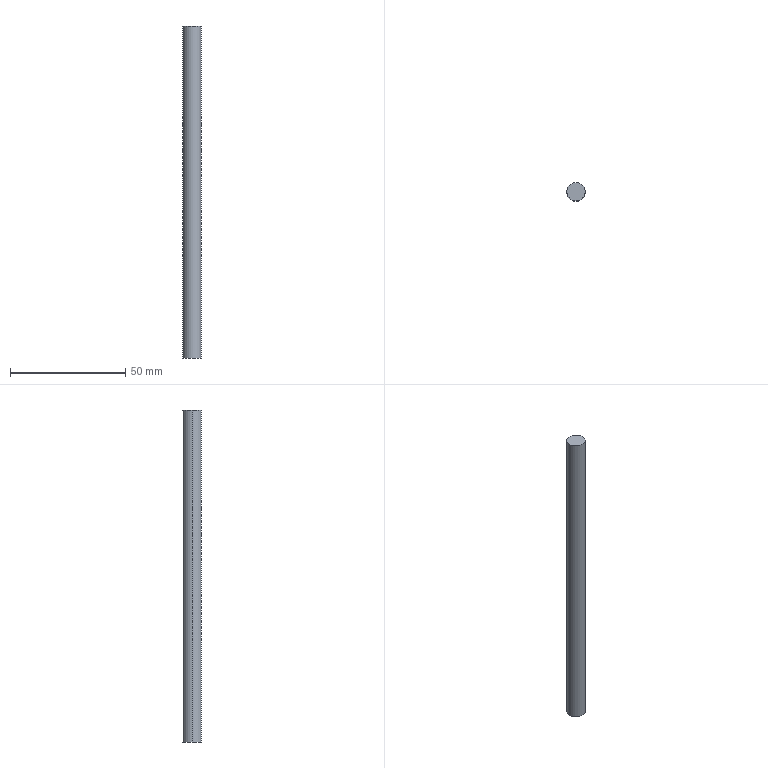Part | SolidWorks | features Extrusion 1 | 1 solid | 4 faces | box 8 x 8 x 144 mm | volume 7238 mm3 | cylinder 2 | plane 2 | commonest cylinder face diameters 8 x2
STEP:
#1=CARTESIAN_POINT('',(4.,0.,72.));
#2=VERTEX_POINT('',#1);
#3=CARTESIAN_POINT('',(-4.,0.,72.));
#4=VERTEX_POINT('',#3);
#5=CARTESIAN_POINT('',(0.,0.,72.));
#6=DIRECTION('',(0.,0.,1.));
#7=DIRECTION('',(1.,0.,0.));
#8=AXIS2_PLACEMENT_3D('',#5,#6,#7);
#9=CIRCLE('',#8,4.);
#10=EDGE_CURVE('',#2,#4,#9,.T.);
#11=ORIENTED_EDGE('',*,*,#10,.F.);
#12=CARTESIAN_POINT('',(4.,0.,-72.));
#13=VERTEX_POINT('',#12);
#14=CARTESIAN_POINT('',(4.,0.,72.));
#15=DIRECTION('',(0.,0.,-1.));
#16=VECTOR('',#15,1000.);
#17=LINE('',#14,#16);
#18=EDGE_CURVE('',#2,#13,#17,.T.);
#19=ORIENTED_EDGE('',*,*,#18,.T.);
#20=CARTESIAN_POINT('',(-4.,0.,-72.));
#21=VERTEX_POINT('',#20);
#22=CARTESIAN_POINT('',(0.,0.,-72.));
#23=DIRECTION('',(0.,0.,1.));
#24=DIRECTION('',(1.,0.,0.));
#25=AXIS2_PLACEMENT_3D('',#22,#23,#24);
#26=CIRCLE('',#25,4.);
#27=EDGE_CURVE('',#13,#21,#26,.T.);
#28=ORIENTED_EDGE('',*,*,#27,.T.);
#29=CARTESIAN_POINT('',(-4.,0.,72.));
#30=DIRECTION('',(0.,0.,-1.));
#31=VECTOR('',#30,1000.);
#32=LINE('',#29,#31);
#33=EDGE_CURVE('',#4,#21,#32,.T.);
#34=ORIENTED_EDGE('',*,*,#33,.F.);
#35=EDGE_LOOP('',(#11,#19,#28,#34));
#36=FACE_OUTER_BOUND('',#35,.T.);
#37=CARTESIAN_POINT('',(0.,0.,72.));
#38=DIRECTION('',(0.,0.,-1.));
#39=DIRECTION('',(-1.,0.,0.));
#40=AXIS2_PLACEMENT_3D('',#37,#38,#39);
#41=CYLINDRICAL_SURFACE('',#40,4.);
#42=ADVANCED_FACE('',(#36),#41,.T.);
#43=ORIENTED_EDGE('',*,*,#18,.F.);
#44=CARTESIAN_POINT('',(0.,0.,72.));
#45=DIRECTION('',(0.,0.,1.));
#46=DIRECTION('',(1.,0.,0.));
#47=AXIS2_PLACEMENT_3D('',#44,#45,#46);
#48=CIRCLE('',#47,4.);
#49=EDGE_CURVE('',#4,#2,#48,.T.);
#50=ORIENTED_EDGE('',*,*,#49,.F.);
#51=ORIENTED_EDGE('',*,*,#33,.T.);
#52=CARTESIAN_POINT('',(0.,0.,-72.));
#53=DIRECTION('',(0.,0.,1.));
#54=DIRECTION('',(1.,0.,0.));
#55=AXIS2_PLACEMENT_3D('',#52,#53,#54);
#56=CIRCLE('',#55,4.);
#57=EDGE_CURVE('',#21,#13,#56,.T.);
#58=ORIENTED_EDGE('',*,*,#57,.T.);
#59=EDGE_LOOP('',(#43,#50,#51,#58));
#60=FACE_OUTER_BOUND('',#59,.T.);
#61=CARTESIAN_POINT('',(0.,0.,72.));
#62=DIRECTION('',(0.,0.,-1.));
#63=DIRECTION('',(-1.,0.,0.));
#64=AXIS2_PLACEMENT_3D('',#61,#62,#63);
#65=CYLINDRICAL_SURFACE('',#64,4.);
#66=ADVANCED_FACE('',(#60),#65,.T.);
#67=ORIENTED_EDGE('',*,*,#49,.T.);
#68=ORIENTED_EDGE('',*,*,#10,.T.);
#69=EDGE_LOOP('',(#67,#68));
#70=FACE_OUTER_BOUND('',#69,.T.);
#71=CARTESIAN_POINT('',(0.,0.,72.));
#72=DIRECTION('',(0.,0.,1.));
#73=DIRECTION('',(1.,0.,0.));
#74=AXIS2_PLACEMENT_3D('',#71,#72,#73);
#75=PLANE('',#74);
#76=ADVANCED_FACE('',(#70),#75,.T.);
#77=ORIENTED_EDGE('',*,*,#57,.F.);
#78=ORIENTED_EDGE('',*,*,#27,.F.);
#79=EDGE_LOOP('',(#77,#78));
#80=FACE_OUTER_BOUND('',#79,.T.);
#81=CARTESIAN_POINT('',(0.,0.,-72.));
#82=DIRECTION('',(0.,0.,1.));
#83=DIRECTION('',(1.,0.,0.));
#84=AXIS2_PLACEMENT_3D('',#81,#82,#83);
#85=PLANE('',#84);
#86=ADVANCED_FACE('',(#80),#85,.F.);
#87=CLOSED_SHELL('',(#42,#66,#76,#86));
#88=MANIFOLD_SOLID_BREP('',#87);
#89=CARTESIAN_POINT('',(0.,0.,0.));
#90=DIRECTION('',(0.,0.,1.));
#91=DIRECTION('',(1.,0.,0.));
#92=AXIS2_PLACEMENT_3D('',#89,#90,#91);
#93=(LENGTH_UNIT()NAMED_UNIT(*)SI_UNIT(.MILLI.,.METRE.));
#94=UNCERTAINTY_MEASURE_WITH_UNIT(LENGTH_MEASURE(0.00001),#93,'','');
#95=(NAMED_UNIT(*)PLANE_ANGLE_UNIT()SI_UNIT($,.RADIAN.));
#96=(NAMED_UNIT(*)SI_UNIT($,.STERADIAN.)SOLID_ANGLE_UNIT());
#97=(GEOMETRIC_REPRESENTATION_CONTEXT(3)GLOBAL_UNCERTAINTY_ASSIGNED_CONTEXT((#94))GLOBAL_UNIT_ASSIGNED_CONTEXT((#93,#95,#96))REPRESENTATION_CONTEXT('',''));
#98=ADVANCED_BREP_SHAPE_REPRESENTATION('',(#88,#92),#97);